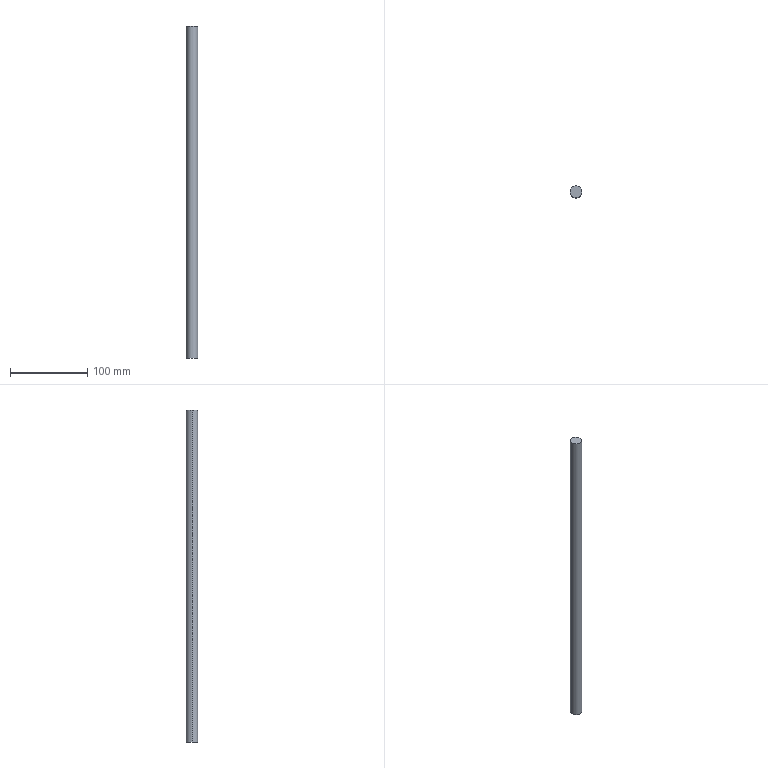Part | SolidWorks | features Extrusion 1 | 1 solid | 4 faces | box 15 x 15 x 430 mm | volume 75987 mm3 | cylinder 2 | plane 2 | commonest cylinder face diameters 15 x2
STEP:
#1=CARTESIAN_POINT('',(7.5,0.,430.));
#2=VERTEX_POINT('',#1);
#3=CARTESIAN_POINT('',(-7.5,0.,430.));
#4=VERTEX_POINT('',#3);
#5=CARTESIAN_POINT('',(0.,0.,430.));
#6=DIRECTION('',(0.,0.,1.));
#7=DIRECTION('',(1.,0.,0.));
#8=AXIS2_PLACEMENT_3D('',#5,#6,#7);
#9=CIRCLE('',#8,7.5);
#10=EDGE_CURVE('',#2,#4,#9,.T.);
#11=ORIENTED_EDGE('',*,*,#10,.F.);
#12=CARTESIAN_POINT('',(7.5,0.,0.));
#13=VERTEX_POINT('',#12);
#14=CARTESIAN_POINT('',(7.5,0.,430.));
#15=DIRECTION('',(0.,0.,-1.));
#16=VECTOR('',#15,1000.);
#17=LINE('',#14,#16);
#18=EDGE_CURVE('',#2,#13,#17,.T.);
#19=ORIENTED_EDGE('',*,*,#18,.T.);
#20=CARTESIAN_POINT('',(-7.5,0.,0.));
#21=VERTEX_POINT('',#20);
#22=CARTESIAN_POINT('',(0.,0.,0.));
#23=DIRECTION('',(0.,0.,1.));
#24=DIRECTION('',(1.,0.,0.));
#25=AXIS2_PLACEMENT_3D('',#22,#23,#24);
#26=CIRCLE('',#25,7.5);
#27=EDGE_CURVE('',#13,#21,#26,.T.);
#28=ORIENTED_EDGE('',*,*,#27,.T.);
#29=CARTESIAN_POINT('',(-7.5,0.,430.));
#30=DIRECTION('',(0.,0.,-1.));
#31=VECTOR('',#30,1000.);
#32=LINE('',#29,#31);
#33=EDGE_CURVE('',#4,#21,#32,.T.);
#34=ORIENTED_EDGE('',*,*,#33,.F.);
#35=EDGE_LOOP('',(#11,#19,#28,#34));
#36=FACE_OUTER_BOUND('',#35,.T.);
#37=CARTESIAN_POINT('',(0.,0.,430.));
#38=DIRECTION('',(0.,0.,-1.));
#39=DIRECTION('',(-1.,0.,0.));
#40=AXIS2_PLACEMENT_3D('',#37,#38,#39);
#41=CYLINDRICAL_SURFACE('',#40,7.5);
#42=ADVANCED_FACE('',(#36),#41,.T.);
#43=ORIENTED_EDGE('',*,*,#18,.F.);
#44=CARTESIAN_POINT('',(0.,0.,430.));
#45=DIRECTION('',(0.,0.,1.));
#46=DIRECTION('',(1.,0.,0.));
#47=AXIS2_PLACEMENT_3D('',#44,#45,#46);
#48=CIRCLE('',#47,7.5);
#49=EDGE_CURVE('',#4,#2,#48,.T.);
#50=ORIENTED_EDGE('',*,*,#49,.F.);
#51=ORIENTED_EDGE('',*,*,#33,.T.);
#52=CARTESIAN_POINT('',(0.,0.,0.));
#53=DIRECTION('',(0.,0.,1.));
#54=DIRECTION('',(1.,0.,0.));
#55=AXIS2_PLACEMENT_3D('',#52,#53,#54);
#56=CIRCLE('',#55,7.5);
#57=EDGE_CURVE('',#21,#13,#56,.T.);
#58=ORIENTED_EDGE('',*,*,#57,.T.);
#59=EDGE_LOOP('',(#43,#50,#51,#58));
#60=FACE_OUTER_BOUND('',#59,.T.);
#61=CARTESIAN_POINT('',(0.,0.,430.));
#62=DIRECTION('',(0.,0.,-1.));
#63=DIRECTION('',(-1.,0.,0.));
#64=AXIS2_PLACEMENT_3D('',#61,#62,#63);
#65=CYLINDRICAL_SURFACE('',#64,7.5);
#66=ADVANCED_FACE('',(#60),#65,.T.);
#67=ORIENTED_EDGE('',*,*,#49,.T.);
#68=ORIENTED_EDGE('',*,*,#10,.T.);
#69=EDGE_LOOP('',(#67,#68));
#70=FACE_OUTER_BOUND('',#69,.T.);
#71=CARTESIAN_POINT('',(0.,0.,430.));
#72=DIRECTION('',(0.,0.,1.));
#73=DIRECTION('',(1.,0.,0.));
#74=AXIS2_PLACEMENT_3D('',#71,#72,#73);
#75=PLANE('',#74);
#76=ADVANCED_FACE('',(#70),#75,.T.);
#77=ORIENTED_EDGE('',*,*,#57,.F.);
#78=ORIENTED_EDGE('',*,*,#27,.F.);
#79=EDGE_LOOP('',(#77,#78));
#80=FACE_OUTER_BOUND('',#79,.T.);
#81=CARTESIAN_POINT('',(0.,0.,0.));
#82=DIRECTION('',(0.,0.,1.));
#83=DIRECTION('',(1.,0.,0.));
#84=AXIS2_PLACEMENT_3D('',#81,#82,#83);
#85=PLANE('',#84);
#86=ADVANCED_FACE('',(#80),#85,.F.);
#87=CLOSED_SHELL('',(#42,#66,#76,#86));
#88=MANIFOLD_SOLID_BREP('',#87);
#89=CARTESIAN_POINT('',(0.,0.,0.));
#90=DIRECTION('',(0.,0.,1.));
#91=DIRECTION('',(1.,0.,0.));
#92=AXIS2_PLACEMENT_3D('',#89,#90,#91);
#93=(LENGTH_UNIT()NAMED_UNIT(*)SI_UNIT(.MILLI.,.METRE.));
#94=UNCERTAINTY_MEASURE_WITH_UNIT(LENGTH_MEASURE(0.00001),#93,'','');
#95=(NAMED_UNIT(*)PLANE_ANGLE_UNIT()SI_UNIT($,.RADIAN.));
#96=(NAMED_UNIT(*)SI_UNIT($,.STERADIAN.)SOLID_ANGLE_UNIT());
#97=(GEOMETRIC_REPRESENTATION_CONTEXT(3)GLOBAL_UNCERTAINTY_ASSIGNED_CONTEXT((#94))GLOBAL_UNIT_ASSIGNED_CONTEXT((#93,#95,#96))REPRESENTATION_CONTEXT('',''));
#98=ADVANCED_BREP_SHAPE_REPRESENTATION('',(#88,#92),#97);